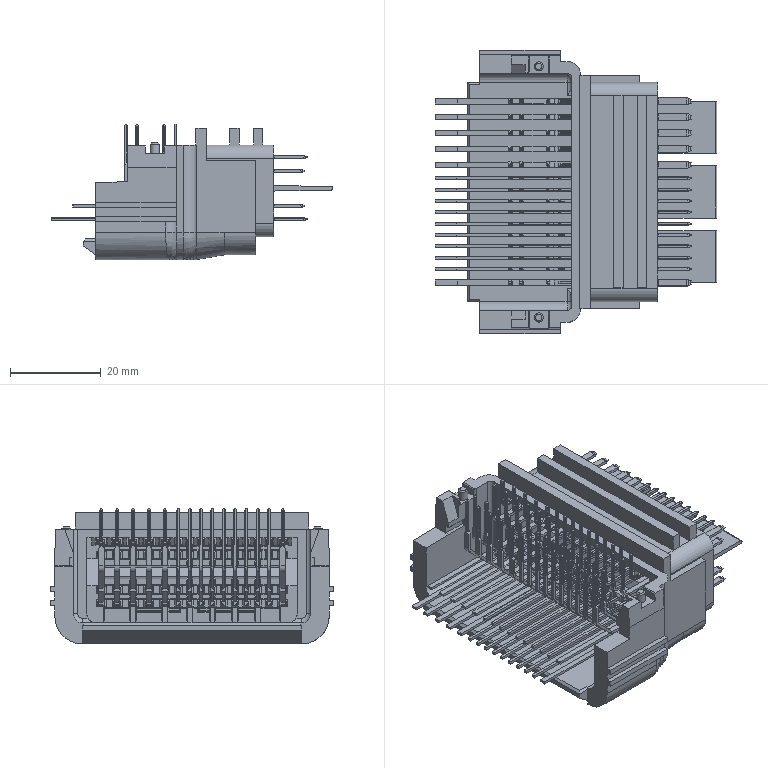Part | NX | features BREP 61 | 85 solids | 21249 faces | volume 27919 mm3 | plane 9057 | cylinder 8477 | torus 1938 | sphere 1505 | spline 268 | cone 4 | commonest cylinder face diameters 0.09 x2464 0.1 x1958 0.2 x1200 2.01 x704 1 x689 0.3 x528